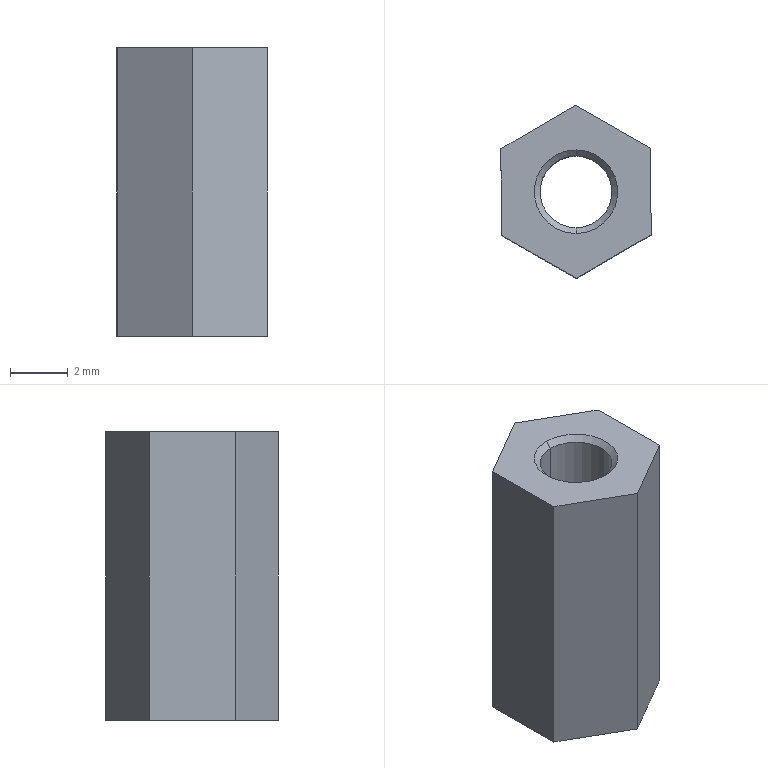Part | SolidWorks | features BaseBody 1 | 1 solid | 14 faces | box 5.209 x 6 x 10 mm | volume 184.409 mm3 | plane 8 | cone 4 | cylinder 2 | commonest cylinder face diameters 2.5 x2
STEP:
#1=CARTESIAN_POINT('',(627.447,-172.298,-73.434));
#2=VERTEX_POINT('',#1);
#3=CARTESIAN_POINT('',(627.447,-169.798,-73.434));
#4=VERTEX_POINT('',#3);
#5=CARTESIAN_POINT('',(627.447,-171.048,-73.434));
#6=DIRECTION('',(-0.000000001,0.000000003,-1.));
#7=DIRECTION('',(0.,1.,0.000000003));
#8=AXIS2_PLACEMENT_3D('',#5,#6,#7);
#9=CIRCLE('',#8,1.25);
#10=EDGE_CURVE('',#2,#4,#9,.T.);
#11=ORIENTED_EDGE('',*,*,#10,.F.);
#12=CARTESIAN_POINT('',(627.447,-172.298,-83.034));
#13=VERTEX_POINT('',#12);
#14=CARTESIAN_POINT('',(627.447,-172.298,-78.234));
#15=DIRECTION('',(-0.000000001,0.000000003,-1.));
#16=VECTOR('',#15,1000.);
#17=LINE('',#14,#16);
#18=EDGE_CURVE('',#2,#13,#17,.T.);
#19=ORIENTED_EDGE('',*,*,#18,.T.);
#20=CARTESIAN_POINT('',(627.447,-169.798,-83.034));
#21=VERTEX_POINT('',#20);
#22=CARTESIAN_POINT('',(627.447,-171.048,-83.034));
#23=DIRECTION('',(0.000000001,-0.000000003,1.));
#24=DIRECTION('',(0.,1.,0.000000003));
#25=AXIS2_PLACEMENT_3D('',#22,#23,#24);
#26=CIRCLE('',#25,1.25);
#27=EDGE_CURVE('',#21,#13,#26,.T.);
#28=ORIENTED_EDGE('',*,*,#27,.F.);
#29=CARTESIAN_POINT('',(627.447,-169.798,-78.234));
#30=DIRECTION('',(-0.000000001,0.000000003,-1.));
#31=VECTOR('',#30,1000.);
#32=LINE('',#29,#31);
#33=EDGE_CURVE('',#4,#21,#32,.T.);
#34=ORIENTED_EDGE('',*,*,#33,.F.);
#35=EDGE_LOOP('',(#11,#19,#28,#34));
#36=FACE_OUTER_BOUND('',#35,.T.);
#37=CARTESIAN_POINT('',(627.447,-171.048,-78.234));
#38=DIRECTION('',(-0.000000001,0.000000003,-1.));
#39=DIRECTION('',(0.,1.,0.000000003));
#40=AXIS2_PLACEMENT_3D('',#37,#38,#39);
#41=CYLINDRICAL_SURFACE('',#40,1.25);
#42=ADVANCED_FACE('',(#36),#41,.F.);
#43=ORIENTED_EDGE('',*,*,#10,.T.);
#44=CARTESIAN_POINT('',(627.447,-169.598,-73.234));
#45=VERTEX_POINT('',#44);
#46=CARTESIAN_POINT('',(627.447,-169.598,-73.234));
#47=DIRECTION('',(0.000000001,0.7071,0.7071));
#48=VECTOR('',#47,1000.);
#49=LINE('',#46,#48);
#50=EDGE_CURVE('',#4,#45,#49,.T.);
#51=ORIENTED_EDGE('',*,*,#50,.T.);
#52=CARTESIAN_POINT('',(627.447,-172.498,-73.234));
#53=VERTEX_POINT('',#52);
#54=CARTESIAN_POINT('',(627.447,-171.048,-73.234));
#55=DIRECTION('',(-0.000000001,0.000000003,-1.));
#56=DIRECTION('',(0.,-1.,-0.000000003));
#57=AXIS2_PLACEMENT_3D('',#54,#55,#56);
#58=CIRCLE('',#57,1.45);
#59=EDGE_CURVE('',#53,#45,#58,.T.);
#60=ORIENTED_EDGE('',*,*,#59,.F.);
#61=CARTESIAN_POINT('',(627.447,-172.498,-73.234));
#62=DIRECTION('',(0.000000001,-0.7071,0.7071));
#63=VECTOR('',#62,1000.);
#64=LINE('',#61,#63);
#65=EDGE_CURVE('',#2,#53,#64,.T.);
#66=ORIENTED_EDGE('',*,*,#65,.F.);
#67=EDGE_LOOP('',(#43,#51,#60,#66));
#68=FACE_OUTER_BOUND('',#67,.T.);
#69=CARTESIAN_POINT('',(627.447,-171.048,-73.234));
#70=DIRECTION('',(0.000000001,-0.000000003,1.));
#71=DIRECTION('',(0.,-1.,-0.000000003));
#72=AXIS2_PLACEMENT_3D('',#69,#70,#71);
#73=CONICAL_SURFACE('',#72,1.45,0.7854);
#74=ADVANCED_FACE('',(#68),#73,.F.);
#75=ORIENTED_EDGE('',*,*,#27,.T.);
#76=CARTESIAN_POINT('',(627.447,-172.498,-83.234));
#77=VERTEX_POINT('',#76);
#78=CARTESIAN_POINT('',(627.447,-172.498,-83.234));
#79=DIRECTION('',(-0.000000001,-0.7071,-0.7071));
#80=VECTOR('',#79,1000.);
#81=LINE('',#78,#80);
#82=EDGE_CURVE('',#13,#77,#81,.T.);
#83=ORIENTED_EDGE('',*,*,#82,.T.);
#84=CARTESIAN_POINT('',(627.447,-169.598,-83.234));
#85=VERTEX_POINT('',#84);
#86=CARTESIAN_POINT('',(627.447,-171.048,-83.234));
#87=DIRECTION('',(0.000000001,-0.000000003,1.));
#88=DIRECTION('',(0.,1.,0.000000003));
#89=AXIS2_PLACEMENT_3D('',#86,#87,#88);
#90=CIRCLE('',#89,1.45);
#91=EDGE_CURVE('',#85,#77,#90,.T.);
#92=ORIENTED_EDGE('',*,*,#91,.F.);
#93=CARTESIAN_POINT('',(627.447,-169.598,-83.234));
#94=DIRECTION('',(-0.000000001,0.7071,-0.7071));
#95=VECTOR('',#94,1000.);
#96=LINE('',#93,#95);
#97=EDGE_CURVE('',#21,#85,#96,.T.);
#98=ORIENTED_EDGE('',*,*,#97,.F.);
#99=EDGE_LOOP('',(#75,#83,#92,#98));
#100=FACE_OUTER_BOUND('',#99,.T.);
#101=CARTESIAN_POINT('',(627.447,-171.048,-83.234));
#102=DIRECTION('',(-0.000000001,0.000000003,-1.));
#103=DIRECTION('',(0.,1.,0.000000003));
#104=AXIS2_PLACEMENT_3D('',#101,#102,#103);
#105=CONICAL_SURFACE('',#104,1.45,0.7854);
#106=ADVANCED_FACE('',(#100),#105,.F.);
#107=ORIENTED_EDGE('',*,*,#18,.F.);
#108=CARTESIAN_POINT('',(627.447,-171.048,-73.434));
#109=DIRECTION('',(-0.000000001,0.000000003,-1.));
#110=DIRECTION('',(0.,1.,0.000000003));
#111=AXIS2_PLACEMENT_3D('',#108,#109,#110);
#112=CIRCLE('',#111,1.25);
#113=EDGE_CURVE('',#4,#2,#112,.T.);
#114=ORIENTED_EDGE('',*,*,#113,.F.);
#115=ORIENTED_EDGE('',*,*,#33,.T.);
#116=CARTESIAN_POINT('',(627.447,-171.048,-83.034));
#117=DIRECTION('',(0.000000001,-0.000000003,1.));
#118=DIRECTION('',(0.,1.,0.000000003));
#119=AXIS2_PLACEMENT_3D('',#116,#117,#118);
#120=CIRCLE('',#119,1.25);
#121=EDGE_CURVE('',#13,#21,#120,.T.);
#122=ORIENTED_EDGE('',*,*,#121,.F.);
#123=EDGE_LOOP('',(#107,#114,#115,#122));
#124=FACE_OUTER_BOUND('',#123,.T.);
#125=CARTESIAN_POINT('',(627.447,-171.048,-78.234));
#126=DIRECTION('',(-0.000000001,0.000000003,-1.));
#127=DIRECTION('',(0.,1.,0.000000003));
#128=AXIS2_PLACEMENT_3D('',#125,#126,#127);
#129=CYLINDRICAL_SURFACE('',#128,1.25);
#130=ADVANCED_FACE('',(#124),#129,.F.);
#131=ORIENTED_EDGE('',*,*,#50,.F.);
#132=ORIENTED_EDGE('',*,*,#113,.T.);
#133=ORIENTED_EDGE('',*,*,#65,.T.);
#134=CARTESIAN_POINT('',(627.447,-171.048,-73.234));
#135=DIRECTION('',(-0.000000001,0.000000003,-1.));
#136=DIRECTION('',(0.,-1.,-0.000000003));
#137=AXIS2_PLACEMENT_3D('',#134,#135,#136);
#138=CIRCLE('',#137,1.45);
#139=EDGE_CURVE('',#45,#53,#138,.T.);
#140=ORIENTED_EDGE('',*,*,#139,.F.);
#141=EDGE_LOOP('',(#131,#132,#133,#140));
#142=FACE_OUTER_BOUND('',#141,.T.);
#143=CARTESIAN_POINT('',(627.447,-171.048,-73.234));
#144=DIRECTION('',(0.000000001,-0.000000003,1.));
#145=DIRECTION('',(0.,-1.,-0.000000003));
#146=AXIS2_PLACEMENT_3D('',#143,#144,#145);
#147=CONICAL_SURFACE('',#146,1.45,0.7854);
#148=ADVANCED_FACE('',(#142),#147,.F.);
#149=ORIENTED_EDGE('',*,*,#82,.F.);
#150=ORIENTED_EDGE('',*,*,#121,.T.);
#151=ORIENTED_EDGE('',*,*,#97,.T.);
#152=CARTESIAN_POINT('',(627.447,-171.048,-83.234));
#153=DIRECTION('',(0.000000001,-0.000000003,1.));
#154=DIRECTION('',(0.,1.,0.000000003));
#155=AXIS2_PLACEMENT_3D('',#152,#153,#154);
#156=CIRCLE('',#155,1.45);
#157=EDGE_CURVE('',#77,#85,#156,.T.);
#158=ORIENTED_EDGE('',*,*,#157,.F.);
#159=EDGE_LOOP('',(#149,#150,#151,#158));
#160=FACE_OUTER_BOUND('',#159,.T.);
#161=CARTESIAN_POINT('',(627.447,-171.048,-83.234));
#162=DIRECTION('',(-0.000000001,0.000000003,-1.));
#163=DIRECTION('',(0.,1.,0.000000003));
#164=AXIS2_PLACEMENT_3D('',#161,#162,#163);
#165=CONICAL_SURFACE('',#164,1.45,0.7854);
#166=ADVANCED_FACE('',(#160),#165,.F.);
#167=ORIENTED_EDGE('',*,*,#59,.T.);
#168=ORIENTED_EDGE('',*,*,#139,.T.);
#169=EDGE_LOOP('',(#167,#168));
#170=FACE_BOUND('',#169,.T.);
#171=CARTESIAN_POINT('',(627.46,-174.048,-73.234));
#172=VERTEX_POINT('',#171);
#173=CARTESIAN_POINT('',(630.051,-172.537,-73.234));
#174=VERTEX_POINT('',#173);
#175=CARTESIAN_POINT('',(627.46,-174.048,-73.234));
#176=DIRECTION('',(0.8638,0.5038,0.000000001));
#177=VECTOR('',#176,1000.);
#178=LINE('',#175,#177);
#179=EDGE_CURVE('',#172,#174,#178,.T.);
#180=ORIENTED_EDGE('',*,*,#179,.T.);
#181=CARTESIAN_POINT('',(630.038,-169.537,-73.234));
#182=VERTEX_POINT('',#181);
#183=CARTESIAN_POINT('',(630.051,-172.537,-73.234));
#184=DIRECTION('',(-0.004352,1.,0.000000003));
#185=VECTOR('',#184,1000.);
#186=LINE('',#183,#185);
#187=EDGE_CURVE('',#174,#182,#186,.T.);
#188=ORIENTED_EDGE('',*,*,#187,.T.);
#189=CARTESIAN_POINT('',(627.434,-168.048,-73.234));
#190=VERTEX_POINT('',#189);
#191=CARTESIAN_POINT('',(630.038,-169.537,-73.234));
#192=DIRECTION('',(-0.8682,0.4962,0.000000002));
#193=VECTOR('',#192,1000.);
#194=LINE('',#191,#193);
#195=EDGE_CURVE('',#182,#190,#194,.T.);
#196=ORIENTED_EDGE('',*,*,#195,.T.);
#197=CARTESIAN_POINT('',(624.842,-169.559,-73.234));
#198=VERTEX_POINT('',#197);
#199=CARTESIAN_POINT('',(627.434,-168.048,-73.234));
#200=DIRECTION('',(-0.8638,-0.5038,-0.000000001));
#201=VECTOR('',#200,1000.);
#202=LINE('',#199,#201);
#203=EDGE_CURVE('',#190,#198,#202,.T.);
#204=ORIENTED_EDGE('',*,*,#203,.T.);
#205=CARTESIAN_POINT('',(624.855,-172.559,-73.234));
#206=VERTEX_POINT('',#205);
#207=CARTESIAN_POINT('',(624.842,-169.559,-73.234));
#208=DIRECTION('',(0.004352,-1.,-0.000000003));
#209=VECTOR('',#208,1000.);
#210=LINE('',#207,#209);
#211=EDGE_CURVE('',#198,#206,#210,.T.);
#212=ORIENTED_EDGE('',*,*,#211,.T.);
#213=CARTESIAN_POINT('',(624.855,-172.559,-73.234));
#214=DIRECTION('',(0.8682,-0.4962,-0.000000002));
#215=VECTOR('',#214,1000.);
#216=LINE('',#213,#215);
#217=EDGE_CURVE('',#206,#172,#216,.T.);
#218=ORIENTED_EDGE('',*,*,#217,.T.);
#219=EDGE_LOOP('',(#180,#188,#196,#204,#212,#218));
#220=FACE_OUTER_BOUND('',#219,.T.);
#221=CARTESIAN_POINT('',(627.447,-171.048,-73.234));
#222=DIRECTION('',(0.000000001,-0.000000003,1.));
#223=DIRECTION('',(0.,-1.,-0.000000003));
#224=AXIS2_PLACEMENT_3D('',#221,#222,#223);
#225=PLANE('',#224);
#226=ADVANCED_FACE('',(#170,#220),#225,.T.);
#227=ORIENTED_EDGE('',*,*,#91,.T.);
#228=ORIENTED_EDGE('',*,*,#157,.T.);
#229=EDGE_LOOP('',(#227,#228));
#230=FACE_BOUND('',#229,.T.);
#231=CARTESIAN_POINT('',(630.038,-169.537,-83.234));
#232=VERTEX_POINT('',#231);
#233=CARTESIAN_POINT('',(627.434,-168.048,-83.234));
#234=VERTEX_POINT('',#233);
#235=CARTESIAN_POINT('',(630.038,-169.537,-83.234));
#236=DIRECTION('',(-0.8682,0.4962,0.000000002));
#237=VECTOR('',#236,1000.);
#238=LINE('',#235,#237);
#239=EDGE_CURVE('',#232,#234,#238,.T.);
#240=ORIENTED_EDGE('',*,*,#239,.F.);
#241=CARTESIAN_POINT('',(630.051,-172.537,-83.234));
#242=VERTEX_POINT('',#241);
#243=CARTESIAN_POINT('',(630.051,-172.537,-83.234));
#244=DIRECTION('',(-0.004352,1.,0.000000003));
#245=VECTOR('',#244,1000.);
#246=LINE('',#243,#245);
#247=EDGE_CURVE('',#242,#232,#246,.T.);
#248=ORIENTED_EDGE('',*,*,#247,.F.);
#249=CARTESIAN_POINT('',(627.46,-174.048,-83.234));
#250=VERTEX_POINT('',#249);
#251=CARTESIAN_POINT('',(627.46,-174.048,-83.234));
#252=DIRECTION('',(0.8638,0.5038,0.000000001));
#253=VECTOR('',#252,1000.);
#254=LINE('',#251,#253);
#255=EDGE_CURVE('',#250,#242,#254,.T.);
#256=ORIENTED_EDGE('',*,*,#255,.F.);
#257=CARTESIAN_POINT('',(624.855,-172.559,-83.234));
#258=VERTEX_POINT('',#257);
#259=CARTESIAN_POINT('',(624.855,-172.559,-83.234));
#260=DIRECTION('',(0.8682,-0.4962,-0.000000002));
#261=VECTOR('',#260,1000.);
#262=LINE('',#259,#261);
#263=EDGE_CURVE('',#258,#250,#262,.T.);
#264=ORIENTED_EDGE('',*,*,#263,.F.);
#265=CARTESIAN_POINT('',(624.842,-169.559,-83.234));
#266=VERTEX_POINT('',#265);
#267=CARTESIAN_POINT('',(624.842,-169.559,-83.234));
#268=DIRECTION('',(0.004352,-1.,-0.000000003));
#269=VECTOR('',#268,1000.);
#270=LINE('',#267,#269);
#271=EDGE_CURVE('',#266,#258,#270,.T.);
#272=ORIENTED_EDGE('',*,*,#271,.F.);
#273=CARTESIAN_POINT('',(627.434,-168.048,-83.234));
#274=DIRECTION('',(-0.8638,-0.5038,-0.000000001));
#275=VECTOR('',#274,1000.);
#276=LINE('',#273,#275);
#277=EDGE_CURVE('',#234,#266,#276,.T.);
#278=ORIENTED_EDGE('',*,*,#277,.F.);
#279=EDGE_LOOP('',(#240,#248,#256,#264,#272,#278));
#280=FACE_OUTER_BOUND('',#279,.T.);
#281=CARTESIAN_POINT('',(627.447,-171.048,-83.234));
#282=DIRECTION('',(0.000000001,-0.000000003,1.));
#283=DIRECTION('',(0.,-1.,-0.000000003));
#284=AXIS2_PLACEMENT_3D('',#281,#282,#283);
#285=PLANE('',#284);
#286=ADVANCED_FACE('',(#230,#280),#285,.F.);
#287=ORIENTED_EDGE('',*,*,#247,.T.);
#288=CARTESIAN_POINT('',(630.038,-169.537,-83.234));
#289=DIRECTION('',(0.000000001,0.,1.));
#290=VECTOR('',#289,1000.);
#291=LINE('',#288,#290);
#292=EDGE_CURVE('',#232,#182,#291,.T.);
#293=ORIENTED_EDGE('',*,*,#292,.T.);
#294=ORIENTED_EDGE('',*,*,#187,.F.);
#295=CARTESIAN_POINT('',(630.051,-172.537,-83.234));
#296=DIRECTION('',(-0.000000001,0.,-1.));
#297=VECTOR('',#296,1000.);
#298=LINE('',#295,#297);
#299=EDGE_CURVE('',#174,#242,#298,.T.);
#300=ORIENTED_EDGE('',*,*,#299,.T.);
#301=EDGE_LOOP('',(#287,#293,#294,#300));
#302=FACE_OUTER_BOUND('',#301,.T.);
#303=CARTESIAN_POINT('',(630.038,-169.537,-83.234));
#304=DIRECTION('',(1.,0.004352,-0.000000001));
#305=DIRECTION('',(-0.004352,1.,0.));
#306=AXIS2_PLACEMENT_3D('',#303,#304,#305);
#307=PLANE('',#306);
#308=ADVANCED_FACE('',(#302),#307,.T.);
#309=ORIENTED_EDGE('',*,*,#255,.T.);
#310=ORIENTED_EDGE('',*,*,#299,.F.);
#311=ORIENTED_EDGE('',*,*,#179,.F.);
#312=CARTESIAN_POINT('',(627.46,-174.048,-83.234));
#313=DIRECTION('',(-0.000000002,0.000000003,-1.));
#314=VECTOR('',#313,1000.);
#315=LINE('',#312,#314);
#316=EDGE_CURVE('',#172,#250,#315,.T.);
#317=ORIENTED_EDGE('',*,*,#316,.T.);
#318=EDGE_LOOP('',(#309,#310,#311,#317));
#319=FACE_OUTER_BOUND('',#318,.T.);
#320=CARTESIAN_POINT('',(630.051,-172.537,-83.234));
#321=DIRECTION('',(0.5038,-0.8638,-0.000000003));
#322=DIRECTION('',(0.8638,0.5038,0.));
#323=AXIS2_PLACEMENT_3D('',#320,#321,#322);
#324=PLANE('',#323);
#325=ADVANCED_FACE('',(#319),#324,.T.);
#326=ORIENTED_EDGE('',*,*,#263,.T.);
#327=ORIENTED_EDGE('',*,*,#316,.F.);
#328=ORIENTED_EDGE('',*,*,#217,.F.);
#329=CARTESIAN_POINT('',(624.855,-172.559,-83.234));
#330=DIRECTION('',(0.000000001,0.000000002,-1.));
#331=VECTOR('',#330,1000.);
#332=LINE('',#329,#331);
#333=EDGE_CURVE('',#206,#258,#332,.T.);
#334=ORIENTED_EDGE('',*,*,#333,.T.);
#335=EDGE_LOOP('',(#326,#327,#328,#334));
#336=FACE_OUTER_BOUND('',#335,.T.);
#337=CARTESIAN_POINT('',(627.46,-174.048,-83.234));
#338=DIRECTION('',(-0.4962,-0.8682,-0.000000003));
#339=DIRECTION('',(0.8682,-0.4962,0.));
#340=AXIS2_PLACEMENT_3D('',#337,#338,#339);
#341=PLANE('',#340);
#342=ADVANCED_FACE('',(#336),#341,.T.);
#343=ORIENTED_EDGE('',*,*,#271,.T.);
#344=ORIENTED_EDGE('',*,*,#333,.F.);
#345=ORIENTED_EDGE('',*,*,#211,.F.);
#346=CARTESIAN_POINT('',(624.842,-169.559,-83.234));
#347=DIRECTION('',(-0.000000001,0.,-1.));
#348=VECTOR('',#347,1000.);
#349=LINE('',#346,#348);
#350=EDGE_CURVE('',#198,#266,#349,.T.);
#351=ORIENTED_EDGE('',*,*,#350,.T.);
#352=EDGE_LOOP('',(#343,#344,#345,#351));
#353=FACE_OUTER_BOUND('',#352,.T.);
#354=CARTESIAN_POINT('',(624.855,-172.559,-83.234));
#355=DIRECTION('',(-1.,-0.004352,0.000000001));
#356=DIRECTION('',(0.004352,-1.,0.));
#357=AXIS2_PLACEMENT_3D('',#354,#355,#356);
#358=PLANE('',#357);
#359=ADVANCED_FACE('',(#353),#358,.T.);
#360=ORIENTED_EDGE('',*,*,#277,.T.);
#361=ORIENTED_EDGE('',*,*,#350,.F.);
#362=ORIENTED_EDGE('',*,*,#203,.F.);
#363=CARTESIAN_POINT('',(627.434,-168.048,-83.234));
#364=DIRECTION('',(-0.000000002,0.000000003,-1.));
#365=VECTOR('',#364,1000.);
#366=LINE('',#363,#365);
#367=EDGE_CURVE('',#190,#234,#366,.T.);
#368=ORIENTED_EDGE('',*,*,#367,.T.);
#369=EDGE_LOOP('',(#360,#361,#362,#368));
#370=FACE_OUTER_BOUND('',#369,.T.);
#371=CARTESIAN_POINT('',(624.842,-169.559,-83.234));
#372=DIRECTION('',(-0.5038,0.8638,0.000000003));
#373=DIRECTION('',(-0.8638,-0.5038,0.));
#374=AXIS2_PLACEMENT_3D('',#371,#372,#373);
#375=PLANE('',#374);
#376=ADVANCED_FACE('',(#370),#375,.T.);
#377=ORIENTED_EDGE('',*,*,#239,.T.);
#378=ORIENTED_EDGE('',*,*,#367,.F.);
#379=ORIENTED_EDGE('',*,*,#195,.F.);
#380=ORIENTED_EDGE('',*,*,#292,.F.);
#381=EDGE_LOOP('',(#377,#378,#379,#380));
#382=FACE_OUTER_BOUND('',#381,.T.);
#383=CARTESIAN_POINT('',(627.434,-168.048,-83.234));
#384=DIRECTION('',(0.4962,0.8682,0.000000003));
#385=DIRECTION('',(-0.8682,0.4962,0.));
#386=AXIS2_PLACEMENT_3D('',#383,#384,#385);
#387=PLANE('',#386);
#388=ADVANCED_FACE('',(#382),#387,.T.);
#389=CLOSED_SHELL('',(#42,#74,#106,#130,#148,#166,#226,#286,#308,#325,#342,#359,#376,#388));
#390=MANIFOLD_SOLID_BREP('',#389);
#391=CARTESIAN_POINT('',(0.,0.,0.));
#392=DIRECTION('',(0.,0.,1.));
#393=DIRECTION('',(1.,0.,0.));
#394=AXIS2_PLACEMENT_3D('',#391,#392,#393);
#395=(LENGTH_UNIT()NAMED_UNIT(*)SI_UNIT(.MILLI.,.METRE.));
#396=UNCERTAINTY_MEASURE_WITH_UNIT(LENGTH_MEASURE(0.00001),#395,'','');
#397=(NAMED_UNIT(*)PLANE_ANGLE_UNIT()SI_UNIT($,.RADIAN.));
#398=(NAMED_UNIT(*)SI_UNIT($,.STERADIAN.)SOLID_ANGLE_UNIT());
#399=(GEOMETRIC_REPRESENTATION_CONTEXT(3)GLOBAL_UNCERTAINTY_ASSIGNED_CONTEXT((#396))GLOBAL_UNIT_ASSIGNED_CONTEXT((#395,#397,#398))REPRESENTATION_CONTEXT('',''));
#400=ADVANCED_BREP_SHAPE_REPRESENTATION('',(#390,#394),#399);